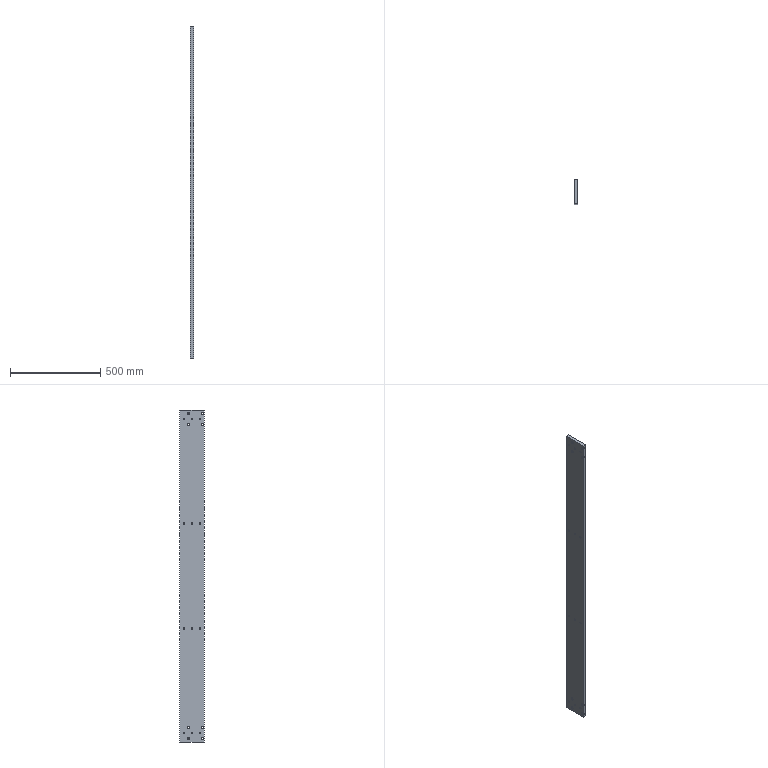Part | SolidWorks | features HoleWzd 2, Extrusion 1, LPattern 1 | 1 solid | 122 faces | box 20 x 136 x 1840 mm | volume 4958995 mm3 | cylinder 80 | plane 26 | cone 16 | commonest cylinder face diameters 9 x40 15 x40